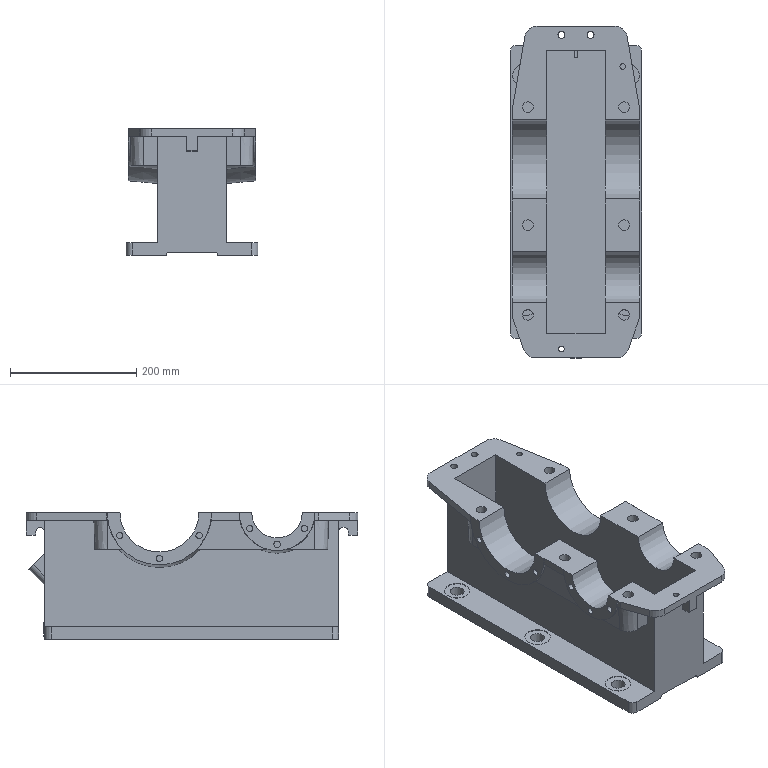Part | NX | features SIMPLE HOLE 56, DATUM_CSYS 27, HOLE PACKAGE 26, SKETCH 26, EXTRUDE 18, EXTRACT_FACE 16, EXTRACT_DATUM_AXIS 10, BLEND 8, CBORE_HOLE 7, EXTRACT_DATUM_PLANE 6, FSET 6, Instance Feature 5, Mirror Feature 5, DRAFT 4, EXTRACT_STRING 2 | 1 solid | 171 faces | box 208 x 525 x 200.222 mm | volume 4335166 mm3 | plane 98 | cylinder 65 | cone 8 | commonest cylinder face diameters 10 x15 40 x10 17 x6 22 x6 32 x6 4 x4